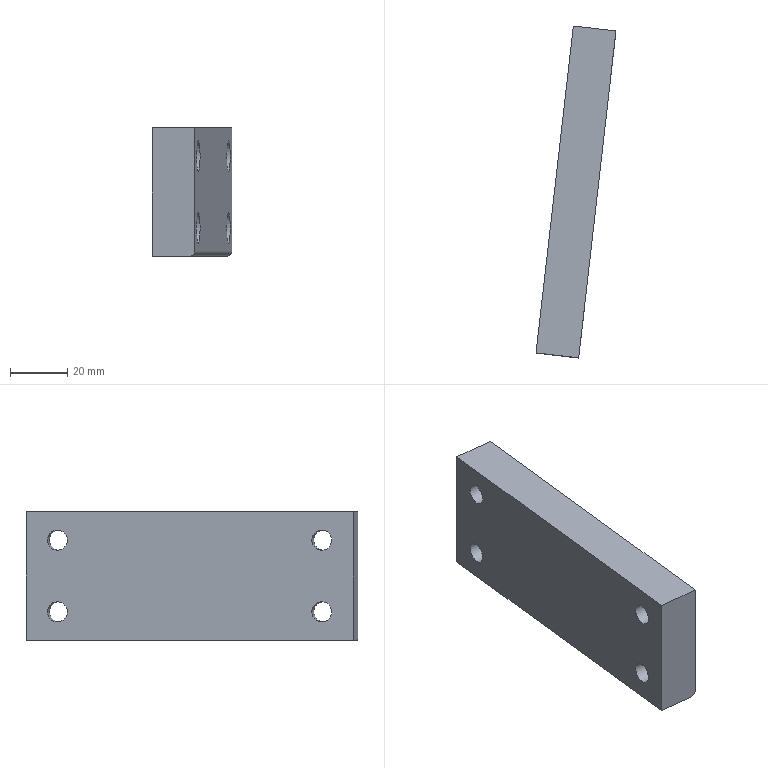Part | NX | features XQ 2 | 1 solid | 19 faces | box 27.922 x 115.959 x 45 mm | volume 73181 mm3 | plane 10 | cylinder 9 | commonest cylinder face diameters 7 x4 11 x4 4 x1
STEP:
#1=CARTESIAN_POINT('',(3451.174,-284.082,-87.));
#2=VERTEX_POINT('',#1);
#3=CARTESIAN_POINT('',(3451.57,-280.604,-87.));
#4=DIRECTION('',(-0.9936,0.1132,0.));
#5=DIRECTION('',(-0.1132,-0.9936,0.));
#6=AXIS2_PLACEMENT_3D('',#3,#4,#5);
#7=CIRCLE('',#6,3.5);
#8=EDGE_CURVE('',#2,#2,#7,.T.);
#9=ORIENTED_EDGE('',*,*,#8,.T.);
#10=EDGE_LOOP('',(#9));
#11=FACE_BOUND('',#10,.T.);
#12=CARTESIAN_POINT('',(3450.948,-286.069,-87.));
#13=VERTEX_POINT('',#12);
#14=CARTESIAN_POINT('',(3451.57,-280.604,-87.));
#15=DIRECTION('',(-0.9936,0.1132,0.));
#16=DIRECTION('',(-0.1132,-0.9936,0.));
#17=AXIS2_PLACEMENT_3D('',#14,#15,#16);
#18=CIRCLE('',#17,5.5);
#19=EDGE_CURVE('',#13,#13,#18,.T.);
#20=ORIENTED_EDGE('',*,*,#19,.F.);
#21=EDGE_LOOP('',(#20));
#22=FACE_BOUND('',#21,.T.);
#23=CARTESIAN_POINT('',(3440.646,-376.484,-5.5));
#24=DIRECTION('',(-0.9936,0.1132,0.));
#25=DIRECTION('',(-0.1132,-0.9936,0.));
#26=AXIS2_PLACEMENT_3D('',#23,#24,#25);
#27=PLANE('',#26);
#28=ADVANCED_FACE('',(#11,#22),#27,.F.);
#29=CARTESIAN_POINT('',(3451.174,-284.082,-62.));
#30=VERTEX_POINT('',#29);
#31=CARTESIAN_POINT('',(3451.57,-280.604,-62.));
#32=DIRECTION('',(0.9936,-0.1132,0.));
#33=DIRECTION('',(-0.1132,-0.9936,0.));
#34=AXIS2_PLACEMENT_3D('',#31,#32,#33);
#35=CIRCLE('',#34,3.5);
#36=EDGE_CURVE('',#30,#30,#35,.T.);
#37=ORIENTED_EDGE('',*,*,#36,.F.);
#38=EDGE_LOOP('',(#37));
#39=FACE_BOUND('',#38,.T.);
#40=CARTESIAN_POINT('',(3450.948,-286.069,-62.));
#41=VERTEX_POINT('',#40);
#42=CARTESIAN_POINT('',(3451.57,-280.604,-62.));
#43=DIRECTION('',(0.9936,-0.1132,0.));
#44=DIRECTION('',(-0.1132,-0.9936,0.));
#45=AXIS2_PLACEMENT_3D('',#42,#43,#44);
#46=CIRCLE('',#45,5.5);
#47=EDGE_CURVE('',#41,#41,#46,.T.);
#48=ORIENTED_EDGE('',*,*,#47,.T.);
#49=EDGE_LOOP('',(#48));
#50=FACE_BOUND('',#49,.T.);
#51=CARTESIAN_POINT('',(3440.646,-376.484,-143.5));
#52=DIRECTION('',(-0.9936,0.1132,0.));
#53=DIRECTION('',(-0.1132,-0.9936,0.));
#54=AXIS2_PLACEMENT_3D('',#51,#52,#53);
#55=PLANE('',#54);
#56=ADVANCED_FACE('',(#39,#50),#55,.F.);
#57=CARTESIAN_POINT('',(3440.646,-376.484,-62.));
#58=VERTEX_POINT('',#57);
#59=CARTESIAN_POINT('',(3441.042,-373.006,-62.));
#60=DIRECTION('',(-0.9936,0.1132,0.));
#61=DIRECTION('',(-0.1132,-0.9936,0.));
#62=AXIS2_PLACEMENT_3D('',#59,#60,#61);
#63=CIRCLE('',#62,3.5);
#64=EDGE_CURVE('',#58,#58,#63,.T.);
#65=ORIENTED_EDGE('',*,*,#64,.T.);
#66=EDGE_LOOP('',(#65));
#67=FACE_BOUND('',#66,.T.);
#68=CARTESIAN_POINT('',(3440.42,-378.471,-62.));
#69=VERTEX_POINT('',#68);
#70=CARTESIAN_POINT('',(3441.042,-373.006,-62.));
#71=DIRECTION('',(-0.9936,0.1132,0.));
#72=DIRECTION('',(-0.1132,-0.9936,0.));
#73=AXIS2_PLACEMENT_3D('',#70,#71,#72);
#74=CIRCLE('',#73,5.5);
#75=EDGE_CURVE('',#69,#69,#74,.T.);
#76=ORIENTED_EDGE('',*,*,#75,.F.);
#77=EDGE_LOOP('',(#76));
#78=FACE_BOUND('',#77,.T.);
#79=CARTESIAN_POINT('',(3451.966,-277.127,-143.5));
#80=DIRECTION('',(-0.9936,0.1132,0.));
#81=DIRECTION('',(0.1132,0.9936,0.));
#82=AXIS2_PLACEMENT_3D('',#79,#80,#81);
#83=PLANE('',#82);
#84=ADVANCED_FACE('',(#67,#78),#83,.F.);
#85=ORIENTED_EDGE('',*,*,#75,.T.);
#86=EDGE_LOOP('',(#85));
#87=FACE_BOUND('',#86,.T.);
#88=CARTESIAN_POINT('',(3449.362,-379.49,-62.));
#89=VERTEX_POINT('',#88);
#90=CARTESIAN_POINT('',(3449.984,-374.025,-62.));
#91=DIRECTION('',(-0.9936,0.1132,0.));
#92=DIRECTION('',(-0.1132,-0.9936,0.));
#93=AXIS2_PLACEMENT_3D('',#90,#91,#92);
#94=CIRCLE('',#93,5.5);
#95=EDGE_CURVE('',#89,#89,#94,.T.);
#96=ORIENTED_EDGE('',*,*,#95,.F.);
#97=EDGE_LOOP('',(#96));
#98=FACE_BOUND('',#97,.T.);
#99=CARTESIAN_POINT('',(3449.984,-374.025,-62.));
#100=DIRECTION('',(-0.9936,0.1132,0.));
#101=DIRECTION('',(0.01966,0.1725,-0.9848));
#102=AXIS2_PLACEMENT_3D('',#99,#100,#101);
#103=CYLINDRICAL_SURFACE('',#102,5.5);
#104=ADVANCED_FACE('',(#87,#98),#103,.F.);
#105=ORIENTED_EDGE('',*,*,#47,.F.);
#106=EDGE_LOOP('',(#105));
#107=FACE_BOUND('',#106,.T.);
#108=CARTESIAN_POINT('',(3459.89,-287.088,-62.));
#109=VERTEX_POINT('',#108);
#110=CARTESIAN_POINT('',(3460.512,-281.623,-62.));
#111=DIRECTION('',(0.9936,-0.1132,0.));
#112=DIRECTION('',(-0.1132,-0.9936,0.));
#113=AXIS2_PLACEMENT_3D('',#110,#111,#112);
#114=CIRCLE('',#113,5.5);
#115=EDGE_CURVE('',#109,#109,#114,.T.);
#116=ORIENTED_EDGE('',*,*,#115,.T.);
#117=EDGE_LOOP('',(#116));
#118=FACE_BOUND('',#117,.T.);
#119=CARTESIAN_POINT('',(3460.512,-281.623,-62.));
#120=DIRECTION('',(-0.9936,0.1132,0.));
#121=DIRECTION('',(-0.01966,-0.1725,-0.9848));
#122=AXIS2_PLACEMENT_3D('',#119,#120,#121);
#123=CYLINDRICAL_SURFACE('',#122,5.5);
#124=ADVANCED_FACE('',(#107,#118),#123,.F.);
#125=ORIENTED_EDGE('',*,*,#19,.T.);
#126=EDGE_LOOP('',(#125));
#127=FACE_BOUND('',#126,.T.);
#128=CARTESIAN_POINT('',(3459.89,-287.088,-87.));
#129=VERTEX_POINT('',#128);
#130=CARTESIAN_POINT('',(3460.512,-281.623,-87.));
#131=DIRECTION('',(-0.9936,0.1132,0.));
#132=DIRECTION('',(-0.1132,-0.9936,0.));
#133=AXIS2_PLACEMENT_3D('',#130,#131,#132);
#134=CIRCLE('',#133,5.5);
#135=EDGE_CURVE('',#129,#129,#134,.T.);
#136=ORIENTED_EDGE('',*,*,#135,.F.);
#137=EDGE_LOOP('',(#136));
#138=FACE_BOUND('',#137,.T.);
#139=CARTESIAN_POINT('',(3460.512,-281.623,-87.));
#140=DIRECTION('',(-0.9936,0.1132,0.));
#141=DIRECTION('',(-0.01966,-0.1725,0.9848));
#142=AXIS2_PLACEMENT_3D('',#139,#140,#141);
#143=CYLINDRICAL_SURFACE('',#142,5.5);
#144=ADVANCED_FACE('',(#127,#138),#143,.F.);
#145=CARTESIAN_POINT('',(3448.739,-384.955,-95.));
#146=VERTEX_POINT('',#145);
#147=CARTESIAN_POINT('',(3461.758,-270.694,-95.));
#148=VERTEX_POINT('',#147);
#149=CARTESIAN_POINT('',(3455.531,-325.34,-95.));
#150=DIRECTION('',(0.1132,0.9936,0.));
#151=VECTOR('',#150,1000.);
#152=LINE('',#149,#151);
#153=EDGE_CURVE('',#146,#148,#152,.T.);
#154=ORIENTED_EDGE('',*,*,#153,.F.);
#155=CARTESIAN_POINT('',(3446.752,-384.728,-97.));
#156=VERTEX_POINT('',#155);
#157=CARTESIAN_POINT('',(3446.752,-384.728,-95.));
#158=DIRECTION('',(0.1132,0.9936,0.));
#159=DIRECTION('',(-0.9936,0.1132,0.));
#160=AXIS2_PLACEMENT_3D('',#157,#158,#159);
#161=CIRCLE('',#160,2.);
#162=EDGE_CURVE('',#146,#156,#161,.T.);
#163=ORIENTED_EDGE('',*,*,#162,.T.);
#164=CARTESIAN_POINT('',(3459.77,-270.467,-97.));
#165=VERTEX_POINT('',#164);
#166=CARTESIAN_POINT('',(3466.094,-214.963,-97.));
#167=DIRECTION('',(-0.1132,-0.9936,0.));
#168=VECTOR('',#167,1000.);
#169=LINE('',#166,#168);
#170=EDGE_CURVE('',#165,#156,#169,.T.);
#171=ORIENTED_EDGE('',*,*,#170,.F.);
#172=CARTESIAN_POINT('',(3459.77,-270.467,-95.));
#173=DIRECTION('',(0.1132,0.9936,0.));
#174=DIRECTION('',(-0.9936,0.1132,0.));
#175=AXIS2_PLACEMENT_3D('',#172,#173,#174);
#176=CIRCLE('',#175,2.);
#177=EDGE_CURVE('',#148,#165,#176,.T.);
#178=ORIENTED_EDGE('',*,*,#177,.F.);
#179=EDGE_LOOP('',(#154,#163,#171,#178));
#180=FACE_BOUND('',#179,.T.);
#181=CARTESIAN_POINT('',(3453.544,-325.114,-95.));
#182=DIRECTION('',(0.1132,0.9936,0.));
#183=DIRECTION('',(-0.9936,0.1132,0.));
#184=AXIS2_PLACEMENT_3D('',#181,#182,#183);
#185=CYLINDRICAL_SURFACE('',#184,2.);
#186=ADVANCED_FACE('',(#180),#185,.T.);
#187=CARTESIAN_POINT('',(3445.213,-283.403,-87.));
#188=VERTEX_POINT('',#187);
#189=CARTESIAN_POINT('',(3445.609,-279.925,-87.));
#190=DIRECTION('',(-0.9936,0.1132,0.));
#191=DIRECTION('',(-0.1132,-0.9936,0.));
#192=AXIS2_PLACEMENT_3D('',#189,#190,#191);
#193=CIRCLE('',#192,3.5);
#194=EDGE_CURVE('',#188,#188,#193,.T.);
#195=ORIENTED_EDGE('',*,*,#194,.T.);
#196=EDGE_LOOP('',(#195));
#197=FACE_BOUND('',#196,.T.);
#198=ORIENTED_EDGE('',*,*,#8,.F.);
#199=EDGE_LOOP('',(#198));
#200=FACE_BOUND('',#199,.T.);
#201=CARTESIAN_POINT('',(3460.512,-281.623,-87.));
#202=DIRECTION('',(-0.9936,0.1132,0.));
#203=DIRECTION('',(-0.01966,-0.1725,0.9848));
#204=AXIS2_PLACEMENT_3D('',#201,#202,#203);
#205=CYLINDRICAL_SURFACE('',#204,3.5);
#206=ADVANCED_FACE('',(#197,#200),#205,.F.);
#207=CARTESIAN_POINT('',(3445.213,-283.403,-62.));
#208=VERTEX_POINT('',#207);
#209=CARTESIAN_POINT('',(3445.609,-279.925,-62.));
#210=DIRECTION('',(-0.9936,0.1132,0.));
#211=DIRECTION('',(-0.1132,-0.9936,0.));
#212=AXIS2_PLACEMENT_3D('',#209,#210,#211);
#213=CIRCLE('',#212,3.5);
#214=EDGE_CURVE('',#208,#208,#213,.T.);
#215=ORIENTED_EDGE('',*,*,#214,.T.);
#216=EDGE_LOOP('',(#215));
#217=FACE_BOUND('',#216,.T.);
#218=ORIENTED_EDGE('',*,*,#36,.T.);
#219=EDGE_LOOP('',(#218));
#220=FACE_BOUND('',#219,.T.);
#221=CARTESIAN_POINT('',(3460.512,-281.623,-62.));
#222=DIRECTION('',(-0.9936,0.1132,0.));
#223=DIRECTION('',(-0.01966,-0.1725,-0.9848));
#224=AXIS2_PLACEMENT_3D('',#221,#222,#223);
#225=CYLINDRICAL_SURFACE('',#224,3.5);
#226=ADVANCED_FACE('',(#217,#220),#225,.F.);
#227=CARTESIAN_POINT('',(3434.685,-375.805,-62.));
#228=VERTEX_POINT('',#227);
#229=CARTESIAN_POINT('',(3435.081,-372.327,-62.));
#230=DIRECTION('',(-0.9936,0.1132,0.));
#231=DIRECTION('',(-0.1132,-0.9936,0.));
#232=AXIS2_PLACEMENT_3D('',#229,#230,#231);
#233=CIRCLE('',#232,3.5);
#234=EDGE_CURVE('',#228,#228,#233,.T.);
#235=ORIENTED_EDGE('',*,*,#234,.T.);
#236=EDGE_LOOP('',(#235));
#237=FACE_BOUND('',#236,.T.);
#238=ORIENTED_EDGE('',*,*,#64,.F.);
#239=EDGE_LOOP('',(#238));
#240=FACE_BOUND('',#239,.T.);
#241=CARTESIAN_POINT('',(3449.984,-374.025,-62.));
#242=DIRECTION('',(-0.9936,0.1132,0.));
#243=DIRECTION('',(0.01966,0.1725,-0.9848));
#244=AXIS2_PLACEMENT_3D('',#241,#242,#243);
#245=CYLINDRICAL_SURFACE('',#244,3.5);
#246=ADVANCED_FACE('',(#237,#240),#245,.F.);
#247=CARTESIAN_POINT('',(3461.758,-270.694,-52.));
#248=VERTEX_POINT('',#247);
#249=CARTESIAN_POINT('',(3461.758,-270.694,-131.));
#250=DIRECTION('',(0.,0.,1.));
#251=VECTOR('',#250,1000.);
#252=LINE('',#249,#251);
#253=EDGE_CURVE('',#148,#248,#252,.T.);
#254=ORIENTED_EDGE('',*,*,#253,.F.);
#255=ORIENTED_EDGE('',*,*,#177,.T.);
#256=CARTESIAN_POINT('',(3446.854,-268.996,-97.));
#257=VERTEX_POINT('',#256);
#258=CARTESIAN_POINT('',(3424.002,-266.392,-97.));
#259=DIRECTION('',(-0.9936,0.1132,0.));
#260=VECTOR('',#259,1000.);
#261=LINE('',#258,#260);
#262=EDGE_CURVE('',#165,#257,#261,.T.);
#263=ORIENTED_EDGE('',*,*,#262,.T.);
#264=CARTESIAN_POINT('',(3446.854,-268.996,-52.));
#265=VERTEX_POINT('',#264);
#266=CARTESIAN_POINT('',(3446.854,-268.996,-15.5));
#267=DIRECTION('',(0.,0.,-1.));
#268=VECTOR('',#267,1000.);
#269=LINE('',#266,#268);
#270=EDGE_CURVE('',#265,#257,#269,.T.);
#271=ORIENTED_EDGE('',*,*,#270,.F.);
#272=CARTESIAN_POINT('',(3464.242,-270.977,-52.));
#273=DIRECTION('',(-0.9936,0.1132,0.));
#274=VECTOR('',#273,1000.);
#275=LINE('',#272,#274);
#276=EDGE_CURVE('',#248,#265,#275,.T.);
#277=ORIENTED_EDGE('',*,*,#276,.F.);
#278=EDGE_LOOP('',(#254,#255,#263,#271,#277));
#279=FACE_BOUND('',#278,.T.);
#280=CARTESIAN_POINT('',(3424.002,-266.392,-75.696));
#281=DIRECTION('',(0.1132,0.9936,0.));
#282=DIRECTION('',(0.,0.,-1.));
#283=AXIS2_PLACEMENT_3D('',#280,#281,#282);
#284=PLANE('',#283);
#285=ADVANCED_FACE('',(#279),#284,.T.);
#286=CARTESIAN_POINT('',(3448.739,-384.955,-52.));
#287=VERTEX_POINT('',#286);
#288=CARTESIAN_POINT('',(3464.196,-249.296,-52.));
#289=DIRECTION('',(0.1132,0.9936,0.));
#290=VECTOR('',#289,1000.);
#291=LINE('',#288,#290);
#292=EDGE_CURVE('',#287,#248,#291,.T.);
#293=ORIENTED_EDGE('',*,*,#292,.T.);
#294=ORIENTED_EDGE('',*,*,#276,.T.);
#295=CARTESIAN_POINT('',(3433.836,-383.257,-52.));
#296=VERTEX_POINT('',#295);
#297=CARTESIAN_POINT('',(3442.043,-311.223,-52.));
#298=DIRECTION('',(0.1132,0.9936,0.));
#299=VECTOR('',#298,1000.);
#300=LINE('',#297,#299);
#301=EDGE_CURVE('',#296,#265,#300,.T.);
#302=ORIENTED_EDGE('',*,*,#301,.F.);
#303=CARTESIAN_POINT('',(3314.217,-369.628,-52.));
#304=DIRECTION('',(0.9936,-0.1132,0.));
#305=VECTOR('',#304,1000.);
#306=LINE('',#303,#305);
#307=EDGE_CURVE('',#296,#287,#306,.T.);
#308=ORIENTED_EDGE('',*,*,#307,.T.);
#309=EDGE_LOOP('',(#293,#294,#302,#308));
#310=FACE_BOUND('',#309,.T.);
#311=CARTESIAN_POINT('',(3466.679,-249.579,-52.));
#312=DIRECTION('',(0.,0.,1.));
#313=DIRECTION('',(0.9588,-0.284,0.));
#314=AXIS2_PLACEMENT_3D('',#311,#312,#313);
#315=PLANE('',#314);
#316=ADVANCED_FACE('',(#310),#315,.T.);
#317=ORIENTED_EDGE('',*,*,#162,.F.);
#318=CARTESIAN_POINT('',(3448.739,-384.955,-148.027));
#319=DIRECTION('',(0.,0.,1.));
#320=VECTOR('',#319,1000.);
#321=LINE('',#318,#320);
#322=EDGE_CURVE('',#146,#287,#321,.T.);
#323=ORIENTED_EDGE('',*,*,#322,.T.);
#324=ORIENTED_EDGE('',*,*,#307,.F.);
#325=CARTESIAN_POINT('',(3433.836,-383.257,-97.));
#326=VERTEX_POINT('',#325);
#327=CARTESIAN_POINT('',(3433.836,-383.257,-148.027));
#328=DIRECTION('',(0.,0.,-1.));
#329=VECTOR('',#328,1000.);
#330=LINE('',#327,#329);
#331=EDGE_CURVE('',#296,#326,#330,.T.);
#332=ORIENTED_EDGE('',*,*,#331,.T.);
#333=CARTESIAN_POINT('',(3396.08,-378.955,-97.));
#334=DIRECTION('',(0.9936,-0.1132,0.));
#335=VECTOR('',#334,1000.);
#336=LINE('',#333,#335);
#337=EDGE_CURVE('',#326,#156,#336,.T.);
#338=ORIENTED_EDGE('',*,*,#337,.T.);
#339=EDGE_LOOP('',(#317,#323,#324,#332,#338));
#340=FACE_BOUND('',#339,.T.);
#341=CARTESIAN_POINT('',(3314.217,-369.628,-148.027));
#342=DIRECTION('',(0.1132,0.9936,0.));
#343=DIRECTION('',(0.,0.,-1.));
#344=AXIS2_PLACEMENT_3D('',#341,#342,#343);
#345=PLANE('',#344);
#346=ADVANCED_FACE('',(#340),#345,.F.);
#347=ORIENTED_EDGE('',*,*,#262,.F.);
#348=ORIENTED_EDGE('',*,*,#170,.T.);
#349=ORIENTED_EDGE('',*,*,#337,.F.);
#350=CARTESIAN_POINT('',(3442.043,-311.223,-97.));
#351=DIRECTION('',(-0.1132,-0.9936,0.));
#352=VECTOR('',#351,1000.);
#353=LINE('',#350,#352);
#354=EDGE_CURVE('',#257,#326,#353,.T.);
#355=ORIENTED_EDGE('',*,*,#354,.F.);
#356=EDGE_LOOP('',(#347,#348,#349,#355));
#357=FACE_BOUND('',#356,.T.);
#358=CARTESIAN_POINT('',(3415.422,-209.19,-97.));
#359=DIRECTION('',(0.,0.,1.));
#360=DIRECTION('',(-0.1132,-0.9936,0.));
#361=AXIS2_PLACEMENT_3D('',#358,#359,#360);
#362=PLANE('',#361);
#363=ADVANCED_FACE('',(#357),#362,.F.);
#364=CARTESIAN_POINT('',(3434.685,-375.805,-87.));
#365=VERTEX_POINT('',#364);
#366=CARTESIAN_POINT('',(3435.081,-372.327,-87.));
#367=DIRECTION('',(-0.9936,0.1132,0.));
#368=DIRECTION('',(-0.1132,-0.9936,0.));
#369=AXIS2_PLACEMENT_3D('',#366,#367,#368);
#370=CIRCLE('',#369,3.5);
#371=EDGE_CURVE('',#365,#365,#370,.T.);
#372=ORIENTED_EDGE('',*,*,#371,.F.);
#373=EDGE_LOOP('',(#372));
#374=FACE_BOUND('',#373,.T.);
#375=ORIENTED_EDGE('',*,*,#354,.T.);
#376=ORIENTED_EDGE('',*,*,#331,.F.);
#377=ORIENTED_EDGE('',*,*,#301,.T.);
#378=ORIENTED_EDGE('',*,*,#270,.T.);
#379=EDGE_LOOP('',(#375,#376,#377,#378));
#380=FACE_BOUND('',#379,.T.);
#381=ORIENTED_EDGE('',*,*,#234,.F.);
#382=EDGE_LOOP('',(#381));
#383=FACE_BOUND('',#382,.T.);
#384=ORIENTED_EDGE('',*,*,#214,.F.);
#385=EDGE_LOOP('',(#384));
#386=FACE_BOUND('',#385,.T.);
#387=ORIENTED_EDGE('',*,*,#194,.F.);
#388=EDGE_LOOP('',(#387));
#389=FACE_BOUND('',#388,.T.);
#390=CARTESIAN_POINT('',(3442.043,-311.223,-15.5));
#391=DIRECTION('',(-0.9936,0.1132,0.));
#392=DIRECTION('',(-0.1132,-0.9936,0.));
#393=AXIS2_PLACEMENT_3D('',#390,#391,#392);
#394=PLANE('',#393);
#395=ADVANCED_FACE('',(#374,#380,#383,#386,#389),#394,.T.);
#396=CARTESIAN_POINT('',(3449.362,-379.49,-87.));
#397=VERTEX_POINT('',#396);
#398=CARTESIAN_POINT('',(3449.984,-374.025,-87.));
#399=DIRECTION('',(-0.9936,0.1132,0.));
#400=DIRECTION('',(-0.1132,-0.9936,0.));
#401=AXIS2_PLACEMENT_3D('',#398,#399,#400);
#402=CIRCLE('',#401,5.5);
#403=EDGE_CURVE('',#397,#397,#402,.T.);
#404=ORIENTED_EDGE('',*,*,#403,.T.);
#405=EDGE_LOOP('',(#404));
#406=FACE_BOUND('',#405,.T.);
#407=ORIENTED_EDGE('',*,*,#322,.F.);
#408=ORIENTED_EDGE('',*,*,#153,.T.);
#409=ORIENTED_EDGE('',*,*,#253,.T.);
#410=ORIENTED_EDGE('',*,*,#292,.F.);
#411=EDGE_LOOP('',(#407,#408,#409,#410));
#412=FACE_BOUND('',#411,.T.);
#413=ORIENTED_EDGE('',*,*,#135,.T.);
#414=EDGE_LOOP('',(#413));
#415=FACE_BOUND('',#414,.T.);
#416=ORIENTED_EDGE('',*,*,#115,.F.);
#417=EDGE_LOOP('',(#416));
#418=FACE_BOUND('',#417,.T.);
#419=ORIENTED_EDGE('',*,*,#95,.T.);
#420=EDGE_LOOP('',(#419));
#421=FACE_BOUND('',#420,.T.);
#422=CARTESIAN_POINT('',(3455.531,-325.34,-131.));
#423=DIRECTION('',(-0.9936,0.1132,0.));
#424=DIRECTION('',(-0.1132,-0.9936,0.));
#425=AXIS2_PLACEMENT_3D('',#422,#423,#424);
#426=PLANE('',#425);
#427=ADVANCED_FACE('',(#406,#412,#415,#418,#421),#426,.F.);
#428=CARTESIAN_POINT('',(3440.646,-376.484,-87.));
#429=VERTEX_POINT('',#428);
#430=CARTESIAN_POINT('',(3441.042,-373.006,-87.));
#431=DIRECTION('',(-0.9936,0.1132,0.));
#432=DIRECTION('',(-0.1132,-0.9936,0.));
#433=AXIS2_PLACEMENT_3D('',#430,#431,#432);
#434=CIRCLE('',#433,3.5);
#435=EDGE_CURVE('',#429,#429,#434,.T.);
#436=ORIENTED_EDGE('',*,*,#435,.T.);
#437=EDGE_LOOP('',(#436));
#438=FACE_BOUND('',#437,.T.);
#439=CARTESIAN_POINT('',(3440.42,-378.471,-87.));
#440=VERTEX_POINT('',#439);
#441=CARTESIAN_POINT('',(3441.042,-373.006,-87.));
#442=DIRECTION('',(-0.9936,0.1132,0.));
#443=DIRECTION('',(-0.1132,-0.9936,0.));
#444=AXIS2_PLACEMENT_3D('',#441,#442,#443);
#445=CIRCLE('',#444,5.5);
#446=EDGE_CURVE('',#440,#440,#445,.T.);
#447=ORIENTED_EDGE('',*,*,#446,.F.);
#448=EDGE_LOOP('',(#447));
#449=FACE_BOUND('',#448,.T.);
#450=CARTESIAN_POINT('',(3451.966,-277.127,-5.5));
#451=DIRECTION('',(-0.9936,0.1132,0.));
#452=DIRECTION('',(0.1132,0.9936,0.));
#453=AXIS2_PLACEMENT_3D('',#450,#451,#452);
#454=PLANE('',#453);
#455=ADVANCED_FACE('',(#438,#449),#454,.F.);
#456=ORIENTED_EDGE('',*,*,#371,.T.);
#457=EDGE_LOOP('',(#456));
#458=FACE_BOUND('',#457,.T.);
#459=ORIENTED_EDGE('',*,*,#435,.F.);
#460=EDGE_LOOP('',(#459));
#461=FACE_BOUND('',#460,.T.);
#462=CARTESIAN_POINT('',(3449.984,-374.025,-87.));
#463=DIRECTION('',(-0.9936,0.1132,0.));
#464=DIRECTION('',(0.01966,0.1725,0.9848));
#465=AXIS2_PLACEMENT_3D('',#462,#463,#464);
#466=CYLINDRICAL_SURFACE('',#465,3.5);
#467=ADVANCED_FACE('',(#458,#461),#466,.F.);
#468=ORIENTED_EDGE('',*,*,#446,.T.);
#469=EDGE_LOOP('',(#468));
#470=FACE_BOUND('',#469,.T.);
#471=ORIENTED_EDGE('',*,*,#403,.F.);
#472=EDGE_LOOP('',(#471));
#473=FACE_BOUND('',#472,.T.);
#474=CARTESIAN_POINT('',(3449.984,-374.025,-87.));
#475=DIRECTION('',(-0.9936,0.1132,0.));
#476=DIRECTION('',(0.01966,0.1725,0.9848));
#477=AXIS2_PLACEMENT_3D('',#474,#475,#476);
#478=CYLINDRICAL_SURFACE('',#477,5.5);
#479=ADVANCED_FACE('',(#470,#473),#478,.F.);
#480=CLOSED_SHELL('',(#28,#56,#84,#104,#124,#144,#186,#206,#226,#246,#285,#316,#346,#363,#395,#427,#455,#467,#479));
#481=MANIFOLD_SOLID_BREP('',#480);
#482=(LENGTH_UNIT()NAMED_UNIT(*)SI_UNIT(.MILLI.,.METRE.));
#483=UNCERTAINTY_MEASURE_WITH_UNIT(LENGTH_MEASURE(0.00001),#482,'','');
#484=(NAMED_UNIT(*)PLANE_ANGLE_UNIT()SI_UNIT($,.RADIAN.));
#485=(NAMED_UNIT(*)SI_UNIT($,.STERADIAN.)SOLID_ANGLE_UNIT());
#486=(GEOMETRIC_REPRESENTATION_CONTEXT(3)GLOBAL_UNCERTAINTY_ASSIGNED_CONTEXT((#483))GLOBAL_UNIT_ASSIGNED_CONTEXT((#482,#484,#485))REPRESENTATION_CONTEXT('',''));
#487=ADVANCED_BREP_SHAPE_REPRESENTATION('',(#481),#486);